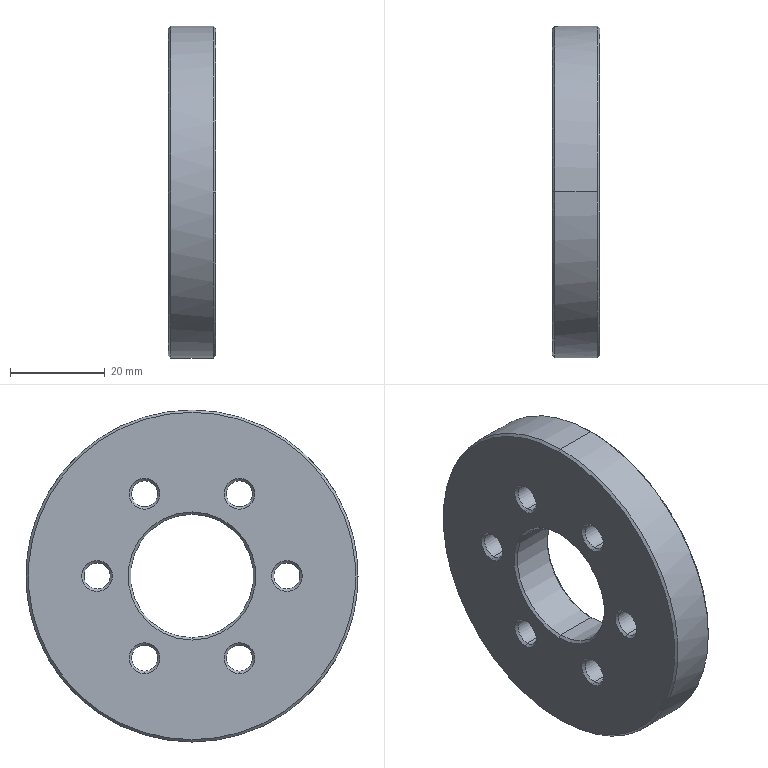Part | STEP file | 05-04 Turntable bottom press plate | 1 solid | 50 faces | box 10 x 70 x 70 mm | volume 31647 mm3 | cone 32 | cylinder 16 | plane 2 | commonest cylinder face diameters 5.5 x12 26 x2 70 x2